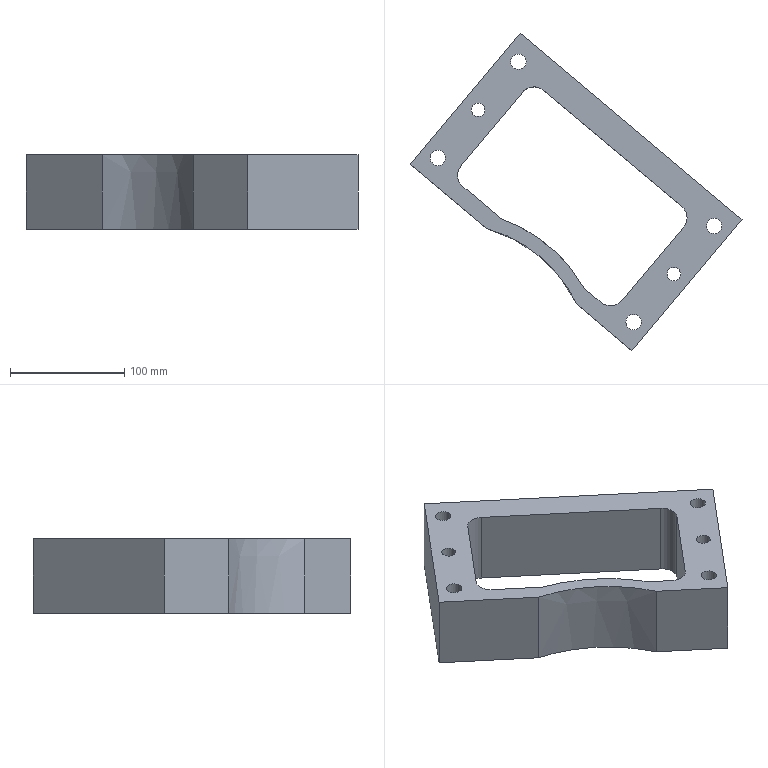Part | NX | features solid 2 | 1 solid | 32 faces | box 290.993 x 278.175 x 65 mm | volume 1076201 mm3 | plane 16 | cylinder 14 | spline 2 | commonest cylinder face diameters 13.5 x4 19.5 x4 26 x4 12 x2
STEP:
#1=CARTESIAN_POINT('',(595.572,489.803,65.));
#2=VERTEX_POINT('',#1);
#3=CARTESIAN_POINT('',(595.572,489.803,0.000000024));
#4=VERTEX_POINT('',#3);
#5=CARTESIAN_POINT('',(595.572,489.803,32.5));
#6=DIRECTION('',(0.,0.,1.));
#7=VECTOR('',#6,1000.);
#8=LINE('',#5,#7);
#9=EDGE_CURVE('',#2,#4,#8,.F.);
#10=ORIENTED_EDGE('',*,*,#9,.F.);
#11=CARTESIAN_POINT('',(610.764,477.056,65.));
#12=VERTEX_POINT('',#11);
#13=CARTESIAN_POINT('',(467.513,597.257,65.));
#14=DIRECTION('',(0.766,-0.6428,0.));
#15=VECTOR('',#14,1000.);
#16=LINE('',#13,#15);
#17=EDGE_CURVE('',#2,#12,#16,.T.);
#18=ORIENTED_EDGE('',*,*,#17,.T.);
#19=CARTESIAN_POINT('',(610.764,477.056,0.000000024));
#20=VERTEX_POINT('',#19);
#21=CARTESIAN_POINT('',(610.764,477.056,70.));
#22=DIRECTION('',(0.,0.,-1.));
#23=VECTOR('',#22,1000.);
#24=LINE('',#21,#23);
#25=EDGE_CURVE('',#20,#12,#24,.F.);
#26=ORIENTED_EDGE('',*,*,#25,.F.);
#27=CARTESIAN_POINT('',(467.513,597.257,0.000000024));
#28=DIRECTION('',(-0.766,0.6428,0.));
#29=VECTOR('',#28,1000.);
#30=LINE('',#27,#29);
#31=EDGE_CURVE('',#4,#20,#30,.F.);
#32=ORIENTED_EDGE('',*,*,#31,.F.);
#33=EDGE_LOOP('',(#10,#18,#26,#32));
#34=FACE_BOUND('',#33,.T.);
#35=CARTESIAN_POINT('',(467.513,597.257,70.));
#36=DIRECTION('',(-0.6428,-0.766,0.));
#37=DIRECTION('',(-0.766,0.6428,0.));
#38=AXIS2_PLACEMENT_3D('',#35,#36,#37);
#39=PLANE('',#38);
#40=ADVANCED_FACE('',(#34),#39,.F.);
#41=CARTESIAN_POINT('',(523.703,550.108,0.000000024));
#42=VERTEX_POINT('',#41);
#43=CARTESIAN_POINT('',(523.703,550.108,65.));
#44=VERTEX_POINT('',#43);
#45=CARTESIAN_POINT('',(523.703,550.108,0.000000024));
#46=DIRECTION('',(0.,0.,1.));
#47=VECTOR('',#46,1000.);
#48=LINE('',#45,#47);
#49=EDGE_CURVE('',#42,#44,#48,.T.);
#50=ORIENTED_EDGE('',*,*,#49,.F.);
#51=CARTESIAN_POINT('',(489.728,578.616,0.000000024));
#52=VERTEX_POINT('',#51);
#53=CARTESIAN_POINT('',(467.513,597.257,0.000000024));
#54=DIRECTION('',(-0.766,0.6428,0.));
#55=VECTOR('',#54,1000.);
#56=LINE('',#53,#55);
#57=EDGE_CURVE('',#52,#42,#56,.F.);
#58=ORIENTED_EDGE('',*,*,#57,.F.);
#59=CARTESIAN_POINT('',(489.728,578.616,65.));
#60=VERTEX_POINT('',#59);
#61=CARTESIAN_POINT('',(489.728,578.616,-5.));
#62=DIRECTION('',(0.,0.,-1.));
#63=VECTOR('',#62,1000.);
#64=LINE('',#61,#63);
#65=EDGE_CURVE('',#60,#52,#64,.T.);
#66=ORIENTED_EDGE('',*,*,#65,.F.);
#67=CARTESIAN_POINT('',(467.513,597.257,65.));
#68=DIRECTION('',(0.766,-0.6428,0.));
#69=VECTOR('',#68,1000.);
#70=LINE('',#67,#69);
#71=EDGE_CURVE('',#60,#44,#70,.T.);
#72=ORIENTED_EDGE('',*,*,#71,.T.);
#73=EDGE_LOOP('',(#50,#58,#66,#72));
#74=FACE_BOUND('',#73,.T.);
#75=CARTESIAN_POINT('',(467.513,597.257,70.));
#76=DIRECTION('',(-0.6428,-0.766,0.));
#77=DIRECTION('',(-0.766,0.6428,0.));
#78=AXIS2_PLACEMENT_3D('',#75,#76,#77);
#79=PLANE('',#78);
#80=ADVANCED_FACE('',(#74),#79,.F.);
#81=CARTESIAN_POINT('',(589.775,475.086,0.000000024));
#82=VERTEX_POINT('',#81);
#83=CARTESIAN_POINT('',(589.775,475.086,65.));
#84=VERTEX_POINT('',#83);
#85=CARTESIAN_POINT('',(589.775,475.086,140.));
#86=CARTESIAN_POINT('',(589.775,475.086,125.));
#87=CARTESIAN_POINT('',(589.775,475.086,110.));
#88=CARTESIAN_POINT('',(589.775,475.086,80.));
#89=CARTESIAN_POINT('',(589.775,475.086,65.));
#90=CARTESIAN_POINT('',(589.775,475.086,20.));
#91=CARTESIAN_POINT('',(589.775,475.086,-10.));
#92=CARTESIAN_POINT('',(589.775,475.086,-40.));
#93=B_SPLINE_CURVE_WITH_KNOTS('',3,(#85,#86,#87,#88,#89,#90,#91,#92),.UNSPECIFIED.,.F.,.F.,(4,2,2,4),(0.,0.25,0.5,1.),.UNSPECIFIED.);
#94=EDGE_CURVE('',#82,#84,#93,.F.);
#95=ORIENTED_EDGE('',*,*,#94,.F.);
#96=CARTESIAN_POINT('',(637.892,434.711,0.000000024));
#97=VERTEX_POINT('',#96);
#98=CARTESIAN_POINT('',(565.395,495.543,0.000000024));
#99=DIRECTION('',(-0.766,0.6428,0.));
#100=VECTOR('',#99,1000.);
#101=LINE('',#98,#100);
#102=EDGE_CURVE('',#82,#97,#101,.F.);
#103=ORIENTED_EDGE('',*,*,#102,.T.);
#104=CARTESIAN_POINT('',(637.892,434.711,65.));
#105=VERTEX_POINT('',#104);
#106=CARTESIAN_POINT('',(637.892,434.711,80.));
#107=DIRECTION('',(0.,0.,1.));
#108=VECTOR('',#107,1000.);
#109=LINE('',#106,#108);
#110=EDGE_CURVE('',#97,#105,#109,.T.);
#111=ORIENTED_EDGE('',*,*,#110,.T.);
#112=CARTESIAN_POINT('',(481.236,566.161,65.));
#113=DIRECTION('',(0.766,-0.6428,0.));
#114=VECTOR('',#113,1000.);
#115=LINE('',#112,#114);
#116=EDGE_CURVE('',#84,#105,#115,.T.);
#117=ORIENTED_EDGE('',*,*,#116,.F.);
#118=EDGE_LOOP('',(#95,#103,#111,#117));
#119=FACE_BOUND('',#118,.T.);
#120=CARTESIAN_POINT('',(565.395,495.543,80.));
#121=DIRECTION('',(0.6428,0.766,0.));
#122=DIRECTION('',(0.766,-0.6428,0.));
#123=AXIS2_PLACEMENT_3D('',#120,#121,#122);
#124=PLANE('',#123);
#125=ADVANCED_FACE('',(#119),#124,.F.);
#126=CARTESIAN_POINT('',(510.282,541.788,65.));
#127=VERTEX_POINT('',#126);
#128=CARTESIAN_POINT('',(510.282,541.788,0.000000024));
#129=VERTEX_POINT('',#128);
#130=CARTESIAN_POINT('',(510.282,541.788,80.));
#131=DIRECTION('',(0.,0.,1.));
#132=VECTOR('',#131,1000.);
#133=LINE('',#130,#132);
#134=EDGE_CURVE('',#127,#129,#133,.F.);
#135=ORIENTED_EDGE('',*,*,#134,.F.);
#136=CARTESIAN_POINT('',(443.317,597.979,65.));
#137=VERTEX_POINT('',#136);
#138=CARTESIAN_POINT('',(481.236,566.161,65.));
#139=DIRECTION('',(0.766,-0.6428,0.));
#140=VECTOR('',#139,1000.);
#141=LINE('',#138,#140);
#142=EDGE_CURVE('',#137,#127,#141,.T.);
#143=ORIENTED_EDGE('',*,*,#142,.F.);
#144=CARTESIAN_POINT('',(443.317,597.979,0.000000024));
#145=VERTEX_POINT('',#144);
#146=CARTESIAN_POINT('',(443.317,597.979,80.));
#147=DIRECTION('',(0.,0.,1.));
#148=VECTOR('',#147,1000.);
#149=LINE('',#146,#148);
#150=EDGE_CURVE('',#145,#137,#149,.T.);
#151=ORIENTED_EDGE('',*,*,#150,.F.);
#152=CARTESIAN_POINT('',(565.395,495.543,0.000000024));
#153=DIRECTION('',(-0.766,0.6428,0.));
#154=VECTOR('',#153,1000.);
#155=LINE('',#152,#154);
#156=EDGE_CURVE('',#145,#129,#155,.F.);
#157=ORIENTED_EDGE('',*,*,#156,.T.);
#158=EDGE_LOOP('',(#135,#143,#151,#157));
#159=FACE_BOUND('',#158,.T.);
#160=CARTESIAN_POINT('',(565.395,495.543,80.));
#161=DIRECTION('',(0.6428,0.766,0.));
#162=DIRECTION('',(0.766,-0.6428,0.));
#163=AXIS2_PLACEMENT_3D('',#160,#161,#162);
#164=PLANE('',#163);
#165=ADVANCED_FACE('',(#159),#164,.F.);
#166=CARTESIAN_POINT('',(589.775,475.086,0.000000024));
#167=CARTESIAN_POINT('',(587.836,479.139,0.000000024));
#168=CARTESIAN_POINT('',(583.553,486.985,0.000000024));
#169=CARTESIAN_POINT('',(575.924,498.063,0.000000024));
#170=CARTESIAN_POINT('',(567.159,508.245,0.000000024));
#171=CARTESIAN_POINT('',(557.474,517.317,0.000000024));
#172=CARTESIAN_POINT('',(546.781,525.352,0.000000024));
#173=CARTESIAN_POINT('',(531.331,534.533,0.000000024));
#174=CARTESIAN_POINT('',(518.946,539.404,0.000000024));
#175=CARTESIAN_POINT('',(510.282,541.788,0.000000024));
#176=B_SPLINE_CURVE_WITH_KNOTS('',3,(#166,#167,#168,#169,#170,#171,#172,#173,#174,#175),.UNSPECIFIED.,.F.,.F.,(4,1,1,1,1,1,1,4),(0.,0.0134,0.0268,0.0402,0.0536,0.067,0.0804,0.1072),.UNSPECIFIED.);
#177=EDGE_CURVE('',#82,#129,#176,.T.);
#178=ORIENTED_EDGE('',*,*,#177,.T.);
#179=ORIENTED_EDGE('',*,*,#156,.F.);
#180=CARTESIAN_POINT('',(539.735,712.886,0.000000024));
#181=VERTEX_POINT('',#180);
#182=CARTESIAN_POINT('',(-69.098,-12.692,0.000000024));
#183=DIRECTION('',(0.6428,0.766,0.));
#184=VECTOR('',#183,1000.);
#185=LINE('',#182,#184);
#186=EDGE_CURVE('',#181,#145,#185,.F.);
#187=ORIENTED_EDGE('',*,*,#186,.F.);
#188=CARTESIAN_POINT('',(734.31,549.618,0.000000024));
#189=VERTEX_POINT('',#188);
#190=CARTESIAN_POINT('',(722.819,559.26,0.000000024));
#191=DIRECTION('',(-0.766,0.6428,0.));
#192=VECTOR('',#191,1000.);
#193=LINE('',#190,#192);
#194=EDGE_CURVE('',#189,#181,#193,.T.);
#195=ORIENTED_EDGE('',*,*,#194,.F.);
#196=CARTESIAN_POINT('',(125.478,-175.96,0.000000024));
#197=DIRECTION('',(0.6428,0.766,0.));
#198=VECTOR('',#197,1000.);
#199=LINE('',#196,#198);
#200=EDGE_CURVE('',#189,#97,#199,.F.);
#201=ORIENTED_EDGE('',*,*,#200,.T.);
#202=ORIENTED_EDGE('',*,*,#102,.F.);
#203=EDGE_LOOP('',(#178,#179,#187,#195,#201,#202));
#204=FACE_BOUND('',#203,.T.);
#205=CARTESIAN_POINT('',(523.703,550.108,0.000000024));
#206=CARTESIAN_POINT('',(531.205,547.402,0.000000024));
#207=CARTESIAN_POINT('',(545.792,540.631,0.000000024));
#208=CARTESIAN_POINT('',(565.448,526.903,0.000000024));
#209=CARTESIAN_POINT('',(582.431,509.864,0.000000024));
#210=CARTESIAN_POINT('',(591.599,496.685,0.000000024));
#211=CARTESIAN_POINT('',(595.572,489.803,0.000000024));
#212=B_SPLINE_CURVE_WITH_KNOTS('',3,(#205,#206,#207,#208,#209,#210,#211),.UNSPECIFIED.,.F.,.F.,(4,1,1,1,4),(0.2128,0.2368,0.2608,0.2847,0.3087),.UNSPECIFIED.);
#213=EDGE_CURVE('',#42,#4,#212,.T.);
#214=ORIENTED_EDGE('',*,*,#213,.T.);
#215=ORIENTED_EDGE('',*,*,#31,.T.);
#216=CARTESIAN_POINT('',(629.078,478.658,0.000000024));
#217=VERTEX_POINT('',#216);
#218=CARTESIAN_POINT('',(619.12,487.014,0.000000024));
#219=DIRECTION('',(0.,0.,-1.));
#220=DIRECTION('',(-1.,0.,0.));
#221=AXIS2_PLACEMENT_3D('',#218,#219,#220);
#222=CIRCLE('',#221,13.);
#223=EDGE_CURVE('',#217,#20,#222,.T.);
#224=ORIENTED_EDGE('',*,*,#223,.F.);
#225=CARTESIAN_POINT('',(683.072,543.006,0.000000024));
#226=VERTEX_POINT('',#225);
#227=CARTESIAN_POINT('',(668.931,526.153,0.000000024));
#228=DIRECTION('',(0.6428,0.766,0.));
#229=VECTOR('',#228,1000.);
#230=LINE('',#227,#229);
#231=EDGE_CURVE('',#226,#217,#230,.F.);
#232=ORIENTED_EDGE('',*,*,#231,.F.);
#233=CARTESIAN_POINT('',(681.47,561.321,0.000000024));
#234=VERTEX_POINT('',#233);
#235=CARTESIAN_POINT('',(673.114,551.362,0.000000024));
#236=DIRECTION('',(0.,0.,-1.));
#237=DIRECTION('',(-1.,0.,0.));
#238=AXIS2_PLACEMENT_3D('',#235,#236,#237);
#239=CIRCLE('',#238,13.);
#240=EDGE_CURVE('',#234,#226,#239,.T.);
#241=ORIENTED_EDGE('',*,*,#240,.F.);
#242=CARTESIAN_POINT('',(560.435,662.881,0.000000024));
#243=VERTEX_POINT('',#242);
#244=CARTESIAN_POINT('',(538.22,681.522,0.000000024));
#245=DIRECTION('',(0.766,-0.6428,0.));
#246=VECTOR('',#245,1000.);
#247=LINE('',#244,#246);
#248=EDGE_CURVE('',#234,#243,#247,.F.);
#249=ORIENTED_EDGE('',*,*,#248,.T.);
#250=CARTESIAN_POINT('',(542.12,661.279,0.000000024));
#251=VERTEX_POINT('',#250);
#252=CARTESIAN_POINT('',(552.079,652.923,0.000000024));
#253=DIRECTION('',(0.,0.,-1.));
#254=DIRECTION('',(-1.,0.,0.));
#255=AXIS2_PLACEMENT_3D('',#252,#253,#254);
#256=CIRCLE('',#255,13.);
#257=EDGE_CURVE('',#251,#243,#256,.T.);
#258=ORIENTED_EDGE('',*,*,#257,.F.);
#259=CARTESIAN_POINT('',(488.126,596.931,0.000000024));
#260=VERTEX_POINT('',#259);
#261=CARTESIAN_POINT('',(527.979,644.426,0.000000024));
#262=DIRECTION('',(0.6428,0.766,0.));
#263=VECTOR('',#262,1000.);
#264=LINE('',#261,#263);
#265=EDGE_CURVE('',#251,#260,#264,.F.);
#266=ORIENTED_EDGE('',*,*,#265,.T.);
#267=CARTESIAN_POINT('',(498.085,588.575,0.000000024));
#268=DIRECTION('',(0.,0.,-1.));
#269=DIRECTION('',(-1.,0.,0.));
#270=AXIS2_PLACEMENT_3D('',#267,#268,#269);
#271=CIRCLE('',#270,13.);
#272=EDGE_CURVE('',#52,#260,#271,.T.);
#273=ORIENTED_EDGE('',*,*,#272,.F.);
#274=ORIENTED_EDGE('',*,*,#57,.T.);
#275=EDGE_LOOP('',(#214,#215,#224,#232,#241,#249,#258,#266,#273,#274));
#276=FACE_BOUND('',#275,.T.);
#277=CARTESIAN_POINT('',(497.016,645.791,0.000000024));
#278=VERTEX_POINT('',#277);
#279=CARTESIAN_POINT('',(503.016,645.791,0.000000024));
#280=DIRECTION('',(0.,0.,-1.));
#281=DIRECTION('',(-1.,0.,0.));
#282=AXIS2_PLACEMENT_3D('',#279,#280,#281);
#283=CIRCLE('',#282,6.);
#284=EDGE_CURVE('',#278,#278,#283,.T.);
#285=ORIENTED_EDGE('',*,*,#284,.F.);
#286=EDGE_LOOP('',(#285));
#287=FACE_BOUND('',#286,.T.);
#288=CARTESIAN_POINT('',(668.61,501.806,0.000000024));
#289=VERTEX_POINT('',#288);
#290=CARTESIAN_POINT('',(674.61,501.806,0.000000024));
#291=DIRECTION('',(0.,0.,-1.));
#292=DIRECTION('',(-1.,0.,0.));
#293=AXIS2_PLACEMENT_3D('',#290,#291,#292);
#294=CIRCLE('',#293,6.);
#295=EDGE_CURVE('',#289,#289,#294,.T.);
#296=ORIENTED_EDGE('',*,*,#295,.F.);
#297=EDGE_LOOP('',(#296));
#298=FACE_BOUND('',#297,.T.);
#299=CARTESIAN_POINT('',(457.913,603.658,0.000000024));
#300=VERTEX_POINT('',#299);
#301=CARTESIAN_POINT('',(467.663,603.658,0.000000024));
#302=DIRECTION('',(0.,0.,-1.));
#303=DIRECTION('',(-1.,0.,0.));
#304=AXIS2_PLACEMENT_3D('',#301,#302,#303);
#305=CIRCLE('',#304,9.75);
#306=EDGE_CURVE('',#300,#300,#305,.T.);
#307=ORIENTED_EDGE('',*,*,#306,.F.);
#308=EDGE_LOOP('',(#307));
#309=FACE_BOUND('',#308,.T.);
#310=CARTESIAN_POINT('',(528.62,687.923,0.000000024));
#311=VERTEX_POINT('',#310);
#312=CARTESIAN_POINT('',(538.37,687.923,0.000000024));
#313=DIRECTION('',(0.,0.,-1.));
#314=DIRECTION('',(-1.,0.,0.));
#315=AXIS2_PLACEMENT_3D('',#312,#313,#314);
#316=CIRCLE('',#315,9.75);
#317=EDGE_CURVE('',#311,#311,#316,.T.);
#318=ORIENTED_EDGE('',*,*,#317,.F.);
#319=EDGE_LOOP('',(#318));
#320=FACE_BOUND('',#319,.T.);
#321=CARTESIAN_POINT('',(700.214,543.939,0.000000024));
#322=VERTEX_POINT('',#321);
#323=CARTESIAN_POINT('',(709.964,543.939,0.000000024));
#324=DIRECTION('',(0.,0.,-1.));
#325=DIRECTION('',(-1.,0.,0.));
#326=AXIS2_PLACEMENT_3D('',#323,#324,#325);
#327=CIRCLE('',#326,9.75);
#328=EDGE_CURVE('',#322,#322,#327,.T.);
#329=ORIENTED_EDGE('',*,*,#328,.F.);
#330=EDGE_LOOP('',(#329));
#331=FACE_BOUND('',#330,.T.);
#332=CARTESIAN_POINT('',(629.507,459.674,0.000000024));
#333=VERTEX_POINT('',#332);
#334=CARTESIAN_POINT('',(639.257,459.674,0.000000024));
#335=DIRECTION('',(0.,0.,-1.));
#336=DIRECTION('',(-1.,0.,0.));
#337=AXIS2_PLACEMENT_3D('',#334,#335,#336);
#338=CIRCLE('',#337,9.75);
#339=EDGE_CURVE('',#333,#333,#338,.T.);
#340=ORIENTED_EDGE('',*,*,#339,.F.);
#341=EDGE_LOOP('',(#340));
#342=FACE_BOUND('',#341,.T.);
#343=CARTESIAN_POINT('',(515.722,654.71,0.000000024));
#344=DIRECTION('',(0.,0.,1.));
#345=DIRECTION('',(-1.,0.,0.));
#346=AXIS2_PLACEMENT_3D('',#343,#344,#345);
#347=PLANE('',#346);
#348=ADVANCED_FACE('',(#204,#276,#287,#298,#309,#320,#331,#342),#347,.F.);
#349=CARTESIAN_POINT('',(510.282,541.788,65.));
#350=CARTESIAN_POINT('',(514.614,540.596,65.));
#351=CARTESIAN_POINT('',(523.093,537.771,65.));
#352=CARTESIAN_POINT('',(535.323,532.174,65.));
#353=CARTESIAN_POINT('',(546.861,525.292,65.));
#354=CARTESIAN_POINT('',(557.469,517.32,65.));
#355=CARTESIAN_POINT('',(567.232,508.177,65.));
#356=CARTESIAN_POINT('',(578.931,494.535,65.));
#357=CARTESIAN_POINT('',(585.897,483.192,65.));
#358=CARTESIAN_POINT('',(589.775,475.086,65.));
#359=B_SPLINE_CURVE_WITH_KNOTS('',3,(#349,#350,#351,#352,#353,#354,#355,#356,#357,#358),.UNSPECIFIED.,.F.,.F.,(4,1,1,1,1,1,1,4),(0.,0.0134,0.02679,0.04019,0.05359,0.06698,0.08038,0.1072),.UNSPECIFIED.);
#360=EDGE_CURVE('',#127,#84,#359,.T.);
#361=ORIENTED_EDGE('',*,*,#360,.T.);
#362=ORIENTED_EDGE('',*,*,#116,.T.);
#363=CARTESIAN_POINT('',(734.31,549.618,65.));
#364=VERTEX_POINT('',#363);
#365=CARTESIAN_POINT('',(644.32,442.372,65.));
#366=DIRECTION('',(-0.6428,-0.766,0.));
#367=VECTOR('',#366,1000.);
#368=LINE('',#365,#367);
#369=EDGE_CURVE('',#364,#105,#368,.T.);
#370=ORIENTED_EDGE('',*,*,#369,.F.);
#371=CARTESIAN_POINT('',(539.735,712.886,65.));
#372=VERTEX_POINT('',#371);
#373=CARTESIAN_POINT('',(577.654,681.068,65.));
#374=DIRECTION('',(0.766,-0.6428,0.));
#375=VECTOR('',#374,1000.);
#376=LINE('',#373,#375);
#377=EDGE_CURVE('',#364,#372,#376,.F.);
#378=ORIENTED_EDGE('',*,*,#377,.T.);
#379=CARTESIAN_POINT('',(449.744,605.64,65.));
#380=DIRECTION('',(-0.6428,-0.766,0.));
#381=VECTOR('',#380,1000.);
#382=LINE('',#379,#381);
#383=EDGE_CURVE('',#372,#137,#382,.T.);
#384=ORIENTED_EDGE('',*,*,#383,.T.);
#385=ORIENTED_EDGE('',*,*,#142,.T.);
#386=EDGE_LOOP('',(#361,#362,#370,#378,#384,#385));
#387=FACE_BOUND('',#386,.T.);
#388=CARTESIAN_POINT('',(595.572,489.803,65.));
#389=CARTESIAN_POINT('',(591.564,496.744,65.));
#390=CARTESIAN_POINT('',(584.685,506.603,65.));
#391=CARTESIAN_POINT('',(574.009,518.313,65.));
#392=CARTESIAN_POINT('',(556.333,534.575,65.));
#393=CARTESIAN_POINT('',(538.673,544.707,65.));
#394=CARTESIAN_POINT('',(523.703,550.108,65.));
#395=B_SPLINE_CURVE_WITH_KNOTS('',3,(#388,#389,#390,#391,#392,#393,#394),.UNSPECIFIED.,.F.,.F.,(4,1,1,1,4),(0.2301,0.2542,0.2662,0.2782,0.3263),.UNSPECIFIED.);
#396=EDGE_CURVE('',#2,#44,#395,.T.);
#397=ORIENTED_EDGE('',*,*,#396,.T.);
#398=ORIENTED_EDGE('',*,*,#71,.F.);
#399=CARTESIAN_POINT('',(488.126,596.931,65.));
#400=VERTEX_POINT('',#399);
#401=CARTESIAN_POINT('',(498.085,588.575,65.));
#402=DIRECTION('',(0.,0.,-1.));
#403=DIRECTION('',(-1.,0.,0.));
#404=AXIS2_PLACEMENT_3D('',#401,#402,#403);
#405=CIRCLE('',#404,13.);
#406=EDGE_CURVE('',#400,#60,#405,.F.);
#407=ORIENTED_EDGE('',*,*,#406,.F.);
#408=CARTESIAN_POINT('',(542.12,661.279,65.));
#409=VERTEX_POINT('',#408);
#410=CARTESIAN_POINT('',(527.979,644.426,65.));
#411=DIRECTION('',(-0.6428,-0.766,0.));
#412=VECTOR('',#411,1000.);
#413=LINE('',#410,#412);
#414=EDGE_CURVE('',#409,#400,#413,.T.);
#415=ORIENTED_EDGE('',*,*,#414,.F.);
#416=CARTESIAN_POINT('',(560.435,662.881,65.));
#417=VERTEX_POINT('',#416);
#418=CARTESIAN_POINT('',(552.079,652.923,65.));
#419=DIRECTION('',(0.,0.,-1.));
#420=DIRECTION('',(-1.,0.,0.));
#421=AXIS2_PLACEMENT_3D('',#418,#419,#420);
#422=CIRCLE('',#421,13.);
#423=EDGE_CURVE('',#417,#409,#422,.F.);
#424=ORIENTED_EDGE('',*,*,#423,.F.);
#425=CARTESIAN_POINT('',(681.47,561.321,65.));
#426=VERTEX_POINT('',#425);
#427=CARTESIAN_POINT('',(538.22,681.522,65.));
#428=DIRECTION('',(-0.766,0.6428,0.));
#429=VECTOR('',#428,1000.);
#430=LINE('',#427,#429);
#431=EDGE_CURVE('',#426,#417,#430,.T.);
#432=ORIENTED_EDGE('',*,*,#431,.F.);
#433=CARTESIAN_POINT('',(683.072,543.006,65.));
#434=VERTEX_POINT('',#433);
#435=CARTESIAN_POINT('',(673.114,551.362,65.));
#436=DIRECTION('',(0.,0.,-1.));
#437=DIRECTION('',(-1.,0.,0.));
#438=AXIS2_PLACEMENT_3D('',#435,#436,#437);
#439=CIRCLE('',#438,13.);
#440=EDGE_CURVE('',#434,#426,#439,.F.);
#441=ORIENTED_EDGE('',*,*,#440,.F.);
#442=CARTESIAN_POINT('',(629.078,478.658,65.));
#443=VERTEX_POINT('',#442);
#444=CARTESIAN_POINT('',(662.503,518.492,65.));
#445=DIRECTION('',(-0.6428,-0.766,0.));
#446=VECTOR('',#445,1000.);
#447=LINE('',#444,#446);
#448=EDGE_CURVE('',#434,#443,#447,.T.);
#449=ORIENTED_EDGE('',*,*,#448,.T.);
#450=CARTESIAN_POINT('',(619.12,487.014,65.));
#451=DIRECTION('',(0.,0.,-1.));
#452=DIRECTION('',(-1.,0.,0.));
#453=AXIS2_PLACEMENT_3D('',#450,#451,#452);
#454=CIRCLE('',#453,13.);
#455=EDGE_CURVE('',#12,#443,#454,.F.);
#456=ORIENTED_EDGE('',*,*,#455,.F.);
#457=ORIENTED_EDGE('',*,*,#17,.F.);
#458=EDGE_LOOP('',(#397,#398,#407,#415,#424,#432,#441,#449,#456,#457));
#459=FACE_BOUND('',#458,.T.);
#460=CARTESIAN_POINT('',(497.016,645.791,65.));
#461=VERTEX_POINT('',#460);
#462=CARTESIAN_POINT('',(503.016,645.791,65.));
#463=DIRECTION('',(0.,0.,-1.));
#464=DIRECTION('',(-1.,0.,0.));
#465=AXIS2_PLACEMENT_3D('',#462,#463,#464);
#466=CIRCLE('',#465,6.);
#467=EDGE_CURVE('',#461,#461,#466,.T.);
#468=ORIENTED_EDGE('',*,*,#467,.T.);
#469=EDGE_LOOP('',(#468));
#470=FACE_BOUND('',#469,.T.);
#471=CARTESIAN_POINT('',(668.61,501.806,65.));
#472=VERTEX_POINT('',#471);
#473=CARTESIAN_POINT('',(674.61,501.806,65.));
#474=DIRECTION('',(0.,0.,-1.));
#475=DIRECTION('',(-1.,0.,0.));
#476=AXIS2_PLACEMENT_3D('',#473,#474,#475);
#477=CIRCLE('',#476,6.);
#478=EDGE_CURVE('',#472,#472,#477,.T.);
#479=ORIENTED_EDGE('',*,*,#478,.T.);
#480=EDGE_LOOP('',(#479));
#481=FACE_BOUND('',#480,.T.);
#482=CARTESIAN_POINT('',(460.913,603.658,65.));
#483=VERTEX_POINT('',#482);
#484=CARTESIAN_POINT('',(467.663,603.658,65.));
#485=DIRECTION('',(0.,0.,-1.));
#486=DIRECTION('',(-1.,0.,0.));
#487=AXIS2_PLACEMENT_3D('',#484,#485,#486);
#488=CIRCLE('',#487,6.75);
#489=EDGE_CURVE('',#483,#483,#488,.T.);
#490=ORIENTED_EDGE('',*,*,#489,.T.);
#491=EDGE_LOOP('',(#490));
#492=FACE_BOUND('',#491,.T.);
#493=CARTESIAN_POINT('',(531.62,687.923,65.));
#494=VERTEX_POINT('',#493);
#495=CARTESIAN_POINT('',(538.37,687.923,65.));
#496=DIRECTION('',(0.,0.,-1.));
#497=DIRECTION('',(-1.,0.,0.));
#498=AXIS2_PLACEMENT_3D('',#495,#496,#497);
#499=CIRCLE('',#498,6.75);
#500=EDGE_CURVE('',#494,#494,#499,.T.);
#501=ORIENTED_EDGE('',*,*,#500,.T.);
#502=EDGE_LOOP('',(#501));
#503=FACE_BOUND('',#502,.T.);
#504=CARTESIAN_POINT('',(703.214,543.939,65.));
#505=VERTEX_POINT('',#504);
#506=CARTESIAN_POINT('',(709.964,543.939,65.));
#507=DIRECTION('',(0.,0.,-1.));
#508=DIRECTION('',(-1.,0.,0.));
#509=AXIS2_PLACEMENT_3D('',#506,#507,#508);
#510=CIRCLE('',#509,6.75);
#511=EDGE_CURVE('',#505,#505,#510,.T.);
#512=ORIENTED_EDGE('',*,*,#511,.T.);
#513=EDGE_LOOP('',(#512));
#514=FACE_BOUND('',#513,.T.);
#515=CARTESIAN_POINT('',(632.507,459.674,65.));
#516=VERTEX_POINT('',#515);
#517=CARTESIAN_POINT('',(639.257,459.674,65.));
#518=DIRECTION('',(0.,0.,-1.));
#519=DIRECTION('',(-1.,0.,0.));
#520=AXIS2_PLACEMENT_3D('',#517,#518,#519);
#521=CIRCLE('',#520,6.75);
#522=EDGE_CURVE('',#516,#516,#521,.T.);
#523=ORIENTED_EDGE('',*,*,#522,.T.);
#524=EDGE_LOOP('',(#523));
#525=FACE_BOUND('',#524,.T.);
#526=CARTESIAN_POINT('',(487.664,573.822,65.));
#527=DIRECTION('',(0.,0.,1.));
#528=DIRECTION('',(0.08716,-0.9962,0.));
#529=AXIS2_PLACEMENT_3D('',#526,#527,#528);
#530=PLANE('',#529);
#531=ADVANCED_FACE('',(#387,#459,#470,#481,#492,#503,#514,#525),#530,.T.);
#532=ORIENTED_EDGE('',*,*,#377,.F.);
#533=CARTESIAN_POINT('',(734.31,549.618,80.));
#534=DIRECTION('',(0.,0.,-1.));
#535=VECTOR('',#534,1000.);
#536=LINE('',#533,#535);
#537=EDGE_CURVE('',#189,#364,#536,.F.);
#538=ORIENTED_EDGE('',*,*,#537,.F.);
#539=ORIENTED_EDGE('',*,*,#194,.T.);
#540=CARTESIAN_POINT('',(539.735,712.886,80.));
#541=DIRECTION('',(0.,0.,-1.));
#542=VECTOR('',#541,1000.);
#543=LINE('',#540,#542);
#544=EDGE_CURVE('',#181,#372,#543,.F.);
#545=ORIENTED_EDGE('',*,*,#544,.T.);
#546=EDGE_LOOP('',(#532,#538,#539,#545));
#547=FACE_BOUND('',#546,.T.);
#548=CARTESIAN_POINT('',(722.819,559.26,0.000000024));
#549=DIRECTION('',(0.6428,0.766,0.));
#550=DIRECTION('',(0.766,-0.6428,0.));
#551=AXIS2_PLACEMENT_3D('',#548,#549,#550);
#552=PLANE('',#551);
#553=ADVANCED_FACE('',(#547),#552,.T.);
#554=ORIENTED_EDGE('',*,*,#110,.F.);
#555=ORIENTED_EDGE('',*,*,#200,.F.);
#556=ORIENTED_EDGE('',*,*,#537,.T.);
#557=ORIENTED_EDGE('',*,*,#369,.T.);
#558=EDGE_LOOP('',(#554,#555,#556,#557));
#559=FACE_BOUND('',#558,.T.);
#560=CARTESIAN_POINT('',(125.478,-175.96,80.));
#561=DIRECTION('',(0.766,-0.6428,0.));
#562=DIRECTION('',(-0.6428,-0.766,0.));
#563=AXIS2_PLACEMENT_3D('',#560,#561,#562);
#564=PLANE('',#563);
#565=ADVANCED_FACE('',(#559),#564,.T.);
#566=ORIENTED_EDGE('',*,*,#544,.F.);
#567=ORIENTED_EDGE('',*,*,#186,.T.);
#568=ORIENTED_EDGE('',*,*,#150,.T.);
#569=ORIENTED_EDGE('',*,*,#383,.F.);
#570=EDGE_LOOP('',(#566,#567,#568,#569));
#571=FACE_BOUND('',#570,.T.);
#572=CARTESIAN_POINT('',(-69.098,-12.692,80.));
#573=DIRECTION('',(0.766,-0.6428,0.));
#574=DIRECTION('',(-0.6428,-0.766,0.));
#575=AXIS2_PLACEMENT_3D('',#572,#573,#574);
#576=PLANE('',#575);
#577=ADVANCED_FACE('',(#571),#576,.F.);
#578=ORIENTED_EDGE('',*,*,#231,.T.);
#579=CARTESIAN_POINT('',(629.078,478.658,100.));
#580=DIRECTION('',(0.,0.,-1.));
#581=VECTOR('',#580,1000.);
#582=LINE('',#579,#581);
#583=EDGE_CURVE('',#443,#217,#582,.T.);
#584=ORIENTED_EDGE('',*,*,#583,.F.);
#585=ORIENTED_EDGE('',*,*,#448,.F.);
#586=CARTESIAN_POINT('',(683.072,543.006,100.));
#587=DIRECTION('',(0.,0.,-1.));
#588=VECTOR('',#587,1000.);
#589=LINE('',#586,#588);
#590=EDGE_CURVE('',#226,#434,#589,.F.);
#591=ORIENTED_EDGE('',*,*,#590,.F.);
#592=EDGE_LOOP('',(#578,#584,#585,#591));
#593=FACE_BOUND('',#592,.T.);
#594=CARTESIAN_POINT('',(662.503,518.492,100.));
#595=DIRECTION('',(-0.766,0.6428,0.));
#596=DIRECTION('',(-0.6428,-0.766,0.));
#597=AXIS2_PLACEMENT_3D('',#594,#595,#596);
#598=PLANE('',#597);
#599=ADVANCED_FACE('',(#593),#598,.T.);
#600=ORIENTED_EDGE('',*,*,#414,.T.);
#601=CARTESIAN_POINT('',(488.126,596.931,80.));
#602=DIRECTION('',(0.,0.,-1.));
#603=VECTOR('',#602,1000.);
#604=LINE('',#601,#603);
#605=EDGE_CURVE('',#260,#400,#604,.F.);
#606=ORIENTED_EDGE('',*,*,#605,.F.);
#607=ORIENTED_EDGE('',*,*,#265,.F.);
#608=CARTESIAN_POINT('',(542.12,661.279,-5.));
#609=DIRECTION('',(0.,0.,-1.));
#610=VECTOR('',#609,1000.);
#611=LINE('',#608,#610);
#612=EDGE_CURVE('',#409,#251,#611,.T.);
#613=ORIENTED_EDGE('',*,*,#612,.F.);
#614=EDGE_LOOP('',(#600,#606,#607,#613));
#615=FACE_BOUND('',#614,.T.);
#616=CARTESIAN_POINT('',(527.979,644.426,0.000000024));
#617=DIRECTION('',(-0.766,0.6428,0.));
#618=DIRECTION('',(0.6428,0.766,0.));
#619=AXIS2_PLACEMENT_3D('',#616,#617,#618);
#620=PLANE('',#619);
#621=ADVANCED_FACE('',(#615),#620,.F.);
#622=ORIENTED_EDGE('',*,*,#248,.F.);
#623=CARTESIAN_POINT('',(681.47,561.321,70.));
#624=DIRECTION('',(0.,0.,-1.));
#625=VECTOR('',#624,1000.);
#626=LINE('',#623,#625);
#627=EDGE_CURVE('',#426,#234,#626,.T.);
#628=ORIENTED_EDGE('',*,*,#627,.F.);
#629=ORIENTED_EDGE('',*,*,#431,.T.);
#630=CARTESIAN_POINT('',(560.435,662.881,80.));
#631=DIRECTION('',(0.,0.,-1.));
#632=VECTOR('',#631,1000.);
#633=LINE('',#630,#632);
#634=EDGE_CURVE('',#243,#417,#633,.F.);
#635=ORIENTED_EDGE('',*,*,#634,.F.);
#636=EDGE_LOOP('',(#622,#628,#629,#635));
#637=FACE_BOUND('',#636,.T.);
#638=CARTESIAN_POINT('',(538.22,681.522,70.));
#639=DIRECTION('',(0.6428,0.766,0.));
#640=DIRECTION('',(0.766,-0.6428,0.));
#641=AXIS2_PLACEMENT_3D('',#638,#639,#640);
#642=PLANE('',#641);
#643=ADVANCED_FACE('',(#637),#642,.F.);
#644=ORIENTED_EDGE('',*,*,#423,.T.);
#645=ORIENTED_EDGE('',*,*,#612,.T.);
#646=ORIENTED_EDGE('',*,*,#257,.T.);
#647=ORIENTED_EDGE('',*,*,#634,.T.);
#648=EDGE_LOOP('',(#644,#645,#646,#647));
#649=FACE_BOUND('',#648,.T.);
#650=CARTESIAN_POINT('',(552.079,652.923,0.000000024));
#651=DIRECTION('',(0.,0.,1.));
#652=DIRECTION('',(-1.,0.,0.));
#653=AXIS2_PLACEMENT_3D('',#650,#651,#652);
#654=CYLINDRICAL_SURFACE('',#653,13.);
#655=ADVANCED_FACE('',(#649),#654,.F.);
#656=ORIENTED_EDGE('',*,*,#440,.T.);
#657=ORIENTED_EDGE('',*,*,#627,.T.);
#658=ORIENTED_EDGE('',*,*,#240,.T.);
#659=ORIENTED_EDGE('',*,*,#590,.T.);
#660=EDGE_LOOP('',(#656,#657,#658,#659));
#661=FACE_BOUND('',#660,.T.);
#662=CARTESIAN_POINT('',(673.114,551.362,70.));
#663=DIRECTION('',(0.,0.,-1.));
#664=DIRECTION('',(1.,0.,0.));
#665=AXIS2_PLACEMENT_3D('',#662,#663,#664);
#666=CYLINDRICAL_SURFACE('',#665,13.);
#667=ADVANCED_FACE('',(#661),#666,.F.);
#668=ORIENTED_EDGE('',*,*,#455,.T.);
#669=ORIENTED_EDGE('',*,*,#583,.T.);
#670=ORIENTED_EDGE('',*,*,#223,.T.);
#671=ORIENTED_EDGE('',*,*,#25,.T.);
#672=EDGE_LOOP('',(#668,#669,#670,#671));
#673=FACE_BOUND('',#672,.T.);
#674=CARTESIAN_POINT('',(619.12,487.014,100.));
#675=DIRECTION('',(0.,0.,-1.));
#676=DIRECTION('',(1.,0.,0.));
#677=AXIS2_PLACEMENT_3D('',#674,#675,#676);
#678=CYLINDRICAL_SURFACE('',#677,13.);
#679=ADVANCED_FACE('',(#673),#678,.F.);
#680=ORIENTED_EDGE('',*,*,#406,.T.);
#681=ORIENTED_EDGE('',*,*,#65,.T.);
#682=ORIENTED_EDGE('',*,*,#272,.T.);
#683=ORIENTED_EDGE('',*,*,#605,.T.);
#684=EDGE_LOOP('',(#680,#681,#682,#683));
#685=FACE_BOUND('',#684,.T.);
#686=CARTESIAN_POINT('',(498.085,588.575,70.));
#687=DIRECTION('',(0.,0.,1.));
#688=DIRECTION('',(-1.,0.,0.));
#689=AXIS2_PLACEMENT_3D('',#686,#687,#688);
#690=CYLINDRICAL_SURFACE('',#689,13.);
#691=ADVANCED_FACE('',(#685),#690,.F.);
#692=ORIENTED_EDGE('',*,*,#522,.F.);
#693=EDGE_LOOP('',(#692));
#694=FACE_BOUND('',#693,.T.);
#695=CARTESIAN_POINT('',(632.507,459.674,40.));
#696=VERTEX_POINT('',#695);
#697=CARTESIAN_POINT('',(639.257,459.674,40.));
#698=DIRECTION('',(0.,0.,-1.));
#699=DIRECTION('',(-1.,0.,0.));
#700=AXIS2_PLACEMENT_3D('',#697,#698,#699);
#701=CIRCLE('',#700,6.75);
#702=EDGE_CURVE('',#696,#696,#701,.T.);
#703=ORIENTED_EDGE('',*,*,#702,.T.);
#704=EDGE_LOOP('',(#703));
#705=FACE_BOUND('',#704,.T.);
#706=CARTESIAN_POINT('',(639.257,459.674,95.));
#707=DIRECTION('',(0.,0.,1.));
#708=DIRECTION('',(-1.,0.,0.));
#709=AXIS2_PLACEMENT_3D('',#706,#707,#708);
#710=CYLINDRICAL_SURFACE('',#709,6.75);
#711=ADVANCED_FACE('',(#694,#705),#710,.F.);
#712=ORIENTED_EDGE('',*,*,#702,.F.);
#713=EDGE_LOOP('',(#712));
#714=FACE_BOUND('',#713,.T.);
#715=CARTESIAN_POINT('',(629.507,459.674,40.));
#716=VERTEX_POINT('',#715);
#717=CARTESIAN_POINT('',(639.257,459.674,40.));
#718=DIRECTION('',(0.,0.,-1.));
#719=DIRECTION('',(-1.,0.,0.));
#720=AXIS2_PLACEMENT_3D('',#717,#718,#719);
#721=CIRCLE('',#720,9.75);
#722=EDGE_CURVE('',#716,#716,#721,.T.);
#723=ORIENTED_EDGE('',*,*,#722,.T.);
#724=EDGE_LOOP('',(#723));
#725=FACE_BOUND('',#724,.T.);
#726=CARTESIAN_POINT('',(639.257,459.674,40.));
#727=DIRECTION('',(0.,0.,1.));
#728=DIRECTION('',(-1.,0.,0.));
#729=AXIS2_PLACEMENT_3D('',#726,#727,#728);
#730=PLANE('',#729);
#731=ADVANCED_FACE('',(#714,#725),#730,.F.);
#732=ORIENTED_EDGE('',*,*,#722,.F.);
#733=EDGE_LOOP('',(#732));
#734=FACE_BOUND('',#733,.T.);
#735=ORIENTED_EDGE('',*,*,#339,.T.);
#736=EDGE_LOOP('',(#735));
#737=FACE_BOUND('',#736,.T.);
#738=CARTESIAN_POINT('',(639.257,459.674,-5.));
#739=DIRECTION('',(0.,0.,1.));
#740=DIRECTION('',(-1.,0.,0.));
#741=AXIS2_PLACEMENT_3D('',#738,#739,#740);
#742=CYLINDRICAL_SURFACE('',#741,9.75);
#743=ADVANCED_FACE('',(#734,#737),#742,.F.);
#744=ORIENTED_EDGE('',*,*,#511,.F.);
#745=EDGE_LOOP('',(#744));
#746=FACE_BOUND('',#745,.T.);
#747=CARTESIAN_POINT('',(703.214,543.939,40.));
#748=VERTEX_POINT('',#747);
#749=CARTESIAN_POINT('',(709.964,543.939,40.));
#750=DIRECTION('',(0.,0.,-1.));
#751=DIRECTION('',(-1.,0.,0.));
#752=AXIS2_PLACEMENT_3D('',#749,#750,#751);
#753=CIRCLE('',#752,6.75);
#754=EDGE_CURVE('',#748,#748,#753,.T.);
#755=ORIENTED_EDGE('',*,*,#754,.T.);
#756=EDGE_LOOP('',(#755));
#757=FACE_BOUND('',#756,.T.);
#758=CARTESIAN_POINT('',(709.964,543.939,95.));
#759=DIRECTION('',(0.,0.,1.));
#760=DIRECTION('',(-1.,0.,0.));
#761=AXIS2_PLACEMENT_3D('',#758,#759,#760);
#762=CYLINDRICAL_SURFACE('',#761,6.75);
#763=ADVANCED_FACE('',(#746,#757),#762,.F.);
#764=ORIENTED_EDGE('',*,*,#754,.F.);
#765=EDGE_LOOP('',(#764));
#766=FACE_BOUND('',#765,.T.);
#767=CARTESIAN_POINT('',(700.214,543.939,40.));
#768=VERTEX_POINT('',#767);
#769=CARTESIAN_POINT('',(709.964,543.939,40.));
#770=DIRECTION('',(0.,0.,-1.));
#771=DIRECTION('',(-1.,0.,0.));
#772=AXIS2_PLACEMENT_3D('',#769,#770,#771);
#773=CIRCLE('',#772,9.75);
#774=EDGE_CURVE('',#768,#768,#773,.T.);
#775=ORIENTED_EDGE('',*,*,#774,.T.);
#776=EDGE_LOOP('',(#775));
#777=FACE_BOUND('',#776,.T.);
#778=CARTESIAN_POINT('',(703.536,536.278,40.));
#779=DIRECTION('',(0.,0.,1.));
#780=DIRECTION('',(-1.,0.,0.));
#781=AXIS2_PLACEMENT_3D('',#778,#779,#780);
#782=PLANE('',#781);
#783=ADVANCED_FACE('',(#766,#777),#782,.F.);
#784=ORIENTED_EDGE('',*,*,#774,.F.);
#785=EDGE_LOOP('',(#784));
#786=FACE_BOUND('',#785,.T.);
#787=ORIENTED_EDGE('',*,*,#328,.T.);
#788=EDGE_LOOP('',(#787));
#789=FACE_BOUND('',#788,.T.);
#790=CARTESIAN_POINT('',(709.964,543.939,-5.));
#791=DIRECTION('',(0.,0.,1.));
#792=DIRECTION('',(-1.,0.,0.));
#793=AXIS2_PLACEMENT_3D('',#790,#791,#792);
#794=CYLINDRICAL_SURFACE('',#793,9.75);
#795=ADVANCED_FACE('',(#786,#789),#794,.F.);
#796=ORIENTED_EDGE('',*,*,#500,.F.);
#797=EDGE_LOOP('',(#796));
#798=FACE_BOUND('',#797,.T.);
#799=CARTESIAN_POINT('',(531.62,687.923,40.));
#800=VERTEX_POINT('',#799);
#801=CARTESIAN_POINT('',(538.37,687.923,40.));
#802=DIRECTION('',(0.,0.,-1.));
#803=DIRECTION('',(-1.,0.,0.));
#804=AXIS2_PLACEMENT_3D('',#801,#802,#803);
#805=CIRCLE('',#804,6.75);
#806=EDGE_CURVE('',#800,#800,#805,.T.);
#807=ORIENTED_EDGE('',*,*,#806,.T.);
#808=EDGE_LOOP('',(#807));
#809=FACE_BOUND('',#808,.T.);
#810=CARTESIAN_POINT('',(538.37,687.923,95.));
#811=DIRECTION('',(0.,0.,1.));
#812=DIRECTION('',(-1.,0.,0.));
#813=AXIS2_PLACEMENT_3D('',#810,#811,#812);
#814=CYLINDRICAL_SURFACE('',#813,6.75);
#815=ADVANCED_FACE('',(#798,#809),#814,.F.);
#816=ORIENTED_EDGE('',*,*,#806,.F.);
#817=EDGE_LOOP('',(#816));
#818=FACE_BOUND('',#817,.T.);
#819=CARTESIAN_POINT('',(528.62,687.923,40.));
#820=VERTEX_POINT('',#819);
#821=CARTESIAN_POINT('',(538.37,687.923,40.));
#822=DIRECTION('',(0.,0.,-1.));
#823=DIRECTION('',(-1.,0.,0.));
#824=AXIS2_PLACEMENT_3D('',#821,#822,#823);
#825=CIRCLE('',#824,9.75);
#826=EDGE_CURVE('',#820,#820,#825,.T.);
#827=ORIENTED_EDGE('',*,*,#826,.T.);
#828=EDGE_LOOP('',(#827));
#829=FACE_BOUND('',#828,.T.);
#830=CARTESIAN_POINT('',(531.942,680.263,40.));
#831=DIRECTION('',(0.,0.,1.));
#832=DIRECTION('',(-1.,0.,0.));
#833=AXIS2_PLACEMENT_3D('',#830,#831,#832);
#834=PLANE('',#833);
#835=ADVANCED_FACE('',(#818,#829),#834,.F.);
#836=ORIENTED_EDGE('',*,*,#826,.F.);
#837=EDGE_LOOP('',(#836));
#838=FACE_BOUND('',#837,.T.);
#839=ORIENTED_EDGE('',*,*,#317,.T.);
#840=EDGE_LOOP('',(#839));
#841=FACE_BOUND('',#840,.T.);
#842=CARTESIAN_POINT('',(538.37,687.923,-5.));
#843=DIRECTION('',(0.,0.,1.));
#844=DIRECTION('',(-1.,0.,0.));
#845=AXIS2_PLACEMENT_3D('',#842,#843,#844);
#846=CYLINDRICAL_SURFACE('',#845,9.75);
#847=ADVANCED_FACE('',(#838,#841),#846,.F.);
#848=ORIENTED_EDGE('',*,*,#489,.F.);
#849=EDGE_LOOP('',(#848));
#850=FACE_BOUND('',#849,.T.);
#851=CARTESIAN_POINT('',(460.913,603.658,40.));
#852=VERTEX_POINT('',#851);
#853=CARTESIAN_POINT('',(467.663,603.658,40.));
#854=DIRECTION('',(0.,0.,-1.));
#855=DIRECTION('',(-1.,0.,0.));
#856=AXIS2_PLACEMENT_3D('',#853,#854,#855);
#857=CIRCLE('',#856,6.75);
#858=EDGE_CURVE('',#852,#852,#857,.T.);
#859=ORIENTED_EDGE('',*,*,#858,.T.);
#860=EDGE_LOOP('',(#859));
#861=FACE_BOUND('',#860,.T.);
#862=CARTESIAN_POINT('',(467.663,603.658,95.));
#863=DIRECTION('',(0.,0.,1.));
#864=DIRECTION('',(-1.,0.,0.));
#865=AXIS2_PLACEMENT_3D('',#862,#863,#864);
#866=CYLINDRICAL_SURFACE('',#865,6.75);
#867=ADVANCED_FACE('',(#850,#861),#866,.F.);
#868=ORIENTED_EDGE('',*,*,#858,.F.);
#869=EDGE_LOOP('',(#868));
#870=FACE_BOUND('',#869,.T.);
#871=CARTESIAN_POINT('',(457.913,603.658,40.));
#872=VERTEX_POINT('',#871);
#873=CARTESIAN_POINT('',(467.663,603.658,40.));
#874=DIRECTION('',(0.,0.,-1.));
#875=DIRECTION('',(-1.,0.,0.));
#876=AXIS2_PLACEMENT_3D('',#873,#874,#875);
#877=CIRCLE('',#876,9.75);
#878=EDGE_CURVE('',#872,#872,#877,.T.);
#879=ORIENTED_EDGE('',*,*,#878,.T.);
#880=EDGE_LOOP('',(#879));
#881=FACE_BOUND('',#880,.T.);
#882=CARTESIAN_POINT('',(467.663,603.658,40.));
#883=DIRECTION('',(0.,0.,1.));
#884=DIRECTION('',(-1.,0.,0.));
#885=AXIS2_PLACEMENT_3D('',#882,#883,#884);
#886=PLANE('',#885);
#887=ADVANCED_FACE('',(#870,#881),#886,.F.);
#888=ORIENTED_EDGE('',*,*,#878,.F.);
#889=EDGE_LOOP('',(#888));
#890=FACE_BOUND('',#889,.T.);
#891=ORIENTED_EDGE('',*,*,#306,.T.);
#892=EDGE_LOOP('',(#891));
#893=FACE_BOUND('',#892,.T.);
#894=CARTESIAN_POINT('',(467.663,603.658,-5.));
#895=DIRECTION('',(0.,0.,1.));
#896=DIRECTION('',(-1.,0.,0.));
#897=AXIS2_PLACEMENT_3D('',#894,#895,#896);
#898=CYLINDRICAL_SURFACE('',#897,9.75);
#899=ADVANCED_FACE('',(#890,#893),#898,.F.);
#900=ORIENTED_EDGE('',*,*,#478,.F.);
#901=EDGE_LOOP('',(#900));
#902=FACE_BOUND('',#901,.T.);
#903=ORIENTED_EDGE('',*,*,#295,.T.);
#904=EDGE_LOOP('',(#903));
#905=FACE_BOUND('',#904,.T.);
#906=CARTESIAN_POINT('',(674.61,501.806,-5.));
#907=DIRECTION('',(0.,0.,1.));
#908=DIRECTION('',(-1.,0.,0.));
#909=AXIS2_PLACEMENT_3D('',#906,#907,#908);
#910=CYLINDRICAL_SURFACE('',#909,6.);
#911=ADVANCED_FACE('',(#902,#905),#910,.F.);
#912=ORIENTED_EDGE('',*,*,#467,.F.);
#913=EDGE_LOOP('',(#912));
#914=FACE_BOUND('',#913,.T.);
#915=ORIENTED_EDGE('',*,*,#284,.T.);
#916=EDGE_LOOP('',(#915));
#917=FACE_BOUND('',#916,.T.);
#918=CARTESIAN_POINT('',(503.016,645.791,-5.));
#919=DIRECTION('',(0.,0.,1.));
#920=DIRECTION('',(-1.,0.,0.));
#921=AXIS2_PLACEMENT_3D('',#918,#919,#920);
#922=CYLINDRICAL_SURFACE('',#921,6.);
#923=ADVANCED_FACE('',(#914,#917),#922,.F.);
#924=ORIENTED_EDGE('',*,*,#94,.T.);
#925=ORIENTED_EDGE('',*,*,#360,.F.);
#926=ORIENTED_EDGE('',*,*,#134,.T.);
#927=ORIENTED_EDGE('',*,*,#177,.F.);
#928=EDGE_LOOP('',(#924,#925,#926,#927));
#929=FACE_BOUND('',#928,.T.);
#930=CARTESIAN_POINT('',(589.775,475.086,65.));
#931=CARTESIAN_POINT('',(589.775,475.086,60.));
#932=CARTESIAN_POINT('',(589.775,475.086,55.));
#933=CARTESIAN_POINT('',(589.775,475.086,33.333));
#934=CARTESIAN_POINT('',(589.775,475.086,16.667));
#935=CARTESIAN_POINT('',(589.775,475.086,0.000000024));
#936=CARTESIAN_POINT('',(586.046,482.881,65.));
#937=CARTESIAN_POINT('',(586.046,482.881,60.));
#938=CARTESIAN_POINT('',(586.046,482.881,55.));
#939=CARTESIAN_POINT('',(586.046,482.881,33.333));
#940=CARTESIAN_POINT('',(586.046,482.881,16.667));
#941=CARTESIAN_POINT('',(586.046,482.881,0.000000024));
#942=CARTESIAN_POINT('',(581.377,490.558,65.));
#943=CARTESIAN_POINT('',(581.377,490.558,60.));
#944=CARTESIAN_POINT('',(581.377,490.558,55.));
#945=CARTESIAN_POINT('',(581.377,490.558,33.333));
#946=CARTESIAN_POINT('',(581.377,490.558,16.667));
#947=CARTESIAN_POINT('',(581.377,490.558,0.000000024));
#948=CARTESIAN_POINT('',(575.957,497.625,65.));
#949=CARTESIAN_POINT('',(575.957,497.625,60.));
#950=CARTESIAN_POINT('',(575.957,497.625,55.));
#951=CARTESIAN_POINT('',(575.957,497.625,33.333));
#952=CARTESIAN_POINT('',(575.957,497.625,16.667));
#953=CARTESIAN_POINT('',(575.957,497.625,0.000000024));
#954=CARTESIAN_POINT('',(570.536,504.692,65.));
#955=CARTESIAN_POINT('',(570.536,504.692,60.));
#956=CARTESIAN_POINT('',(570.536,504.692,55.));
#957=CARTESIAN_POINT('',(570.536,504.692,33.333));
#958=CARTESIAN_POINT('',(570.536,504.692,16.667));
#959=CARTESIAN_POINT('',(570.536,504.692,0.000000024));
#960=CARTESIAN_POINT('',(564.397,511.163,65.));
#961=CARTESIAN_POINT('',(564.397,511.163,60.));
#962=CARTESIAN_POINT('',(564.397,511.163,55.));
#963=CARTESIAN_POINT('',(564.397,511.163,33.333));
#964=CARTESIAN_POINT('',(564.397,511.163,16.667));
#965=CARTESIAN_POINT('',(564.397,511.163,0.000000024));
#966=CARTESIAN_POINT('',(557.493,516.986,65.));
#967=CARTESIAN_POINT('',(557.493,516.986,60.));
#968=CARTESIAN_POINT('',(557.493,516.986,55.));
#969=CARTESIAN_POINT('',(557.493,516.986,33.333));
#970=CARTESIAN_POINT('',(557.493,516.986,16.667));
#971=CARTESIAN_POINT('',(557.493,516.986,0.000000024));
#972=CARTESIAN_POINT('',(550.59,522.81,65.));
#973=CARTESIAN_POINT('',(550.59,522.81,60.));
#974=CARTESIAN_POINT('',(550.59,522.81,55.));
#975=CARTESIAN_POINT('',(550.59,522.81,33.333));
#976=CARTESIAN_POINT('',(550.59,522.81,16.667));
#977=CARTESIAN_POINT('',(550.59,522.81,0.000000024));
#978=CARTESIAN_POINT('',(543.012,527.871,65.));
#979=CARTESIAN_POINT('',(543.012,527.871,60.));
#980=CARTESIAN_POINT('',(543.012,527.871,55.));
#981=CARTESIAN_POINT('',(543.012,527.871,33.333));
#982=CARTESIAN_POINT('',(543.012,527.871,16.667));
#983=CARTESIAN_POINT('',(543.012,527.871,0.000000024));
#984=CARTESIAN_POINT('',(535.146,531.992,65.));
#985=CARTESIAN_POINT('',(535.146,531.992,60.));
#986=CARTESIAN_POINT('',(535.146,531.992,55.));
#987=CARTESIAN_POINT('',(535.146,531.992,33.333));
#988=CARTESIAN_POINT('',(535.146,531.992,16.667));
#989=CARTESIAN_POINT('',(535.146,531.992,0.000000024));
#990=CARTESIAN_POINT('',(531.213,534.053,65.));
#991=CARTESIAN_POINT('',(531.213,534.053,60.));
#992=CARTESIAN_POINT('',(531.213,534.053,55.));
#993=CARTESIAN_POINT('',(531.213,534.053,33.333));
#994=CARTESIAN_POINT('',(531.213,534.053,16.667));
#995=CARTESIAN_POINT('',(531.213,534.053,0.000000024));
#996=CARTESIAN_POINT('',(527.158,535.91,65.));
#997=CARTESIAN_POINT('',(527.158,535.91,60.));
#998=CARTESIAN_POINT('',(527.158,535.91,55.));
#999=CARTESIAN_POINT('',(527.158,535.91,33.333));
#1000=CARTESIAN_POINT('',(527.158,535.91,16.667));
#1001=CARTESIAN_POINT('',(527.158,535.91,0.000000024));
#1002=CARTESIAN_POINT('',(523.,537.549,65.));
#1003=CARTESIAN_POINT('',(523.,537.549,60.));
#1004=CARTESIAN_POINT('',(523.,537.549,55.));
#1005=CARTESIAN_POINT('',(523.,537.549,33.333));
#1006=CARTESIAN_POINT('',(523.,537.549,16.667));
#1007=CARTESIAN_POINT('',(523.,537.549,0.000000024));
#1008=CARTESIAN_POINT('',(518.841,539.188,65.));
#1009=CARTESIAN_POINT('',(518.841,539.188,60.));
#1010=CARTESIAN_POINT('',(518.841,539.188,55.));
#1011=CARTESIAN_POINT('',(518.841,539.188,33.333));
#1012=CARTESIAN_POINT('',(518.841,539.188,16.667));
#1013=CARTESIAN_POINT('',(518.841,539.188,0.000000024));
#1014=CARTESIAN_POINT('',(514.549,540.614,65.));
#1015=CARTESIAN_POINT('',(514.549,540.614,60.));
#1016=CARTESIAN_POINT('',(514.549,540.614,55.));
#1017=CARTESIAN_POINT('',(514.549,540.614,33.333));
#1018=CARTESIAN_POINT('',(514.549,540.614,16.667));
#1019=CARTESIAN_POINT('',(514.549,540.614,0.000000024));
#1020=CARTESIAN_POINT('',(510.282,541.788,65.));
#1021=CARTESIAN_POINT('',(510.282,541.788,60.));
#1022=CARTESIAN_POINT('',(510.282,541.788,55.));
#1023=CARTESIAN_POINT('',(510.282,541.788,33.333));
#1024=CARTESIAN_POINT('',(510.282,541.788,16.667));
#1025=CARTESIAN_POINT('',(510.282,541.788,0.000000024));
#1026=B_SPLINE_SURFACE_WITH_KNOTS('',3,3,((#930,#931,#932,#933,#934,#935),(#936,#937,#938,#939,#940,#941),(#942,#943,#944,#945,#946,#947),(#948,#949,#950,#951,#952,#953),(#954,#955,#956,#957,#958,#959),(#960,#961,#962,#963,#964,#965),(#966,#967,#968,#969,#970,#971),(#972,#973,#974,#975,#976,#977),(#978,#979,#980,#981,#982,#983),(#984,#985,#986,#987,#988,#989),(#990,#991,#992,#993,#994,#995),(#996,#997,#998,#999,#1000,#1001),(#1002,#1003,#1004,#1005,#1006,#1007),(#1008,#1009,#1010,#1011,#1012,#1013),(#1014,#1015,#1016,#1017,#1018,#1019),(#1020,#1021,#1022,#1023,#1024,#1025)),.SURF_OF_LINEAR_EXTRUSION.,.F.,.F.,.F.,(4,3,3,3,3,4),(4,2,4),(0.,0.25,0.5,0.75,0.875,1.),(0.4167,0.5,0.7778),.UNSPECIFIED.);
#1027=ADVANCED_FACE('',(#929),#1026,.T.);
#1028=ORIENTED_EDGE('',*,*,#396,.F.);
#1029=ORIENTED_EDGE('',*,*,#9,.T.);
#1030=ORIENTED_EDGE('',*,*,#213,.F.);
#1031=ORIENTED_EDGE('',*,*,#49,.T.);
#1032=EDGE_LOOP('',(#1028,#1029,#1030,#1031));
#1033=FACE_BOUND('',#1032,.T.);
#1034=CARTESIAN_POINT('',(523.703,550.108,0.000000024));
#1035=CARTESIAN_POINT('',(523.703,550.108,65.));
#1036=CARTESIAN_POINT('',(531.233,547.392,0.000000024));
#1037=CARTESIAN_POINT('',(531.233,547.392,65.));
#1038=CARTESIAN_POINT('',(542.036,542.382,0.000000024));
#1039=CARTESIAN_POINT('',(542.036,542.382,65.));
#1040=CARTESIAN_POINT('',(555.597,533.785,0.000000024));
#1041=CARTESIAN_POINT('',(555.597,533.785,65.));
#1042=CARTESIAN_POINT('',(568.47,523.908,0.000000024));
#1043=CARTESIAN_POINT('',(568.47,523.908,65.));
#1044=CARTESIAN_POINT('',(582.535,509.722,0.000000024));
#1045=CARTESIAN_POINT('',(582.535,509.722,65.));
#1046=CARTESIAN_POINT('',(591.647,496.601,0.000000024));
#1047=CARTESIAN_POINT('',(591.647,496.601,65.));
#1048=CARTESIAN_POINT('',(595.572,489.803,0.000000024));
#1049=CARTESIAN_POINT('',(595.572,489.803,65.));
#1050=B_SPLINE_SURFACE_WITH_KNOTS('',3,1,((#1034,#1035),(#1036,#1037),(#1038,#1039),(#1040,#1041),(#1042,#1043),(#1044,#1045),(#1046,#1047),(#1048,#1049)),.SURF_OF_LINEAR_EXTRUSION.,.F.,.F.,.F.,(4,1,1,1,1,4),(2,2),(0.06717,0.283,0.391,0.4989,0.7148,0.9307),(0.,1.),.UNSPECIFIED.);
#1051=ADVANCED_FACE('',(#1033),#1050,.F.);
#1052=CLOSED_SHELL('',(#40,#80,#125,#165,#348,#531,#553,#565,#577,#599,#621,#643,#655,#667,#679,#691,#711,#731,#743,#763,#783,#795,#815,#835,#847,#867,#887,#899,#911,#923,#1027,#1051));
#1053=MANIFOLD_SOLID_BREP('',#1052);
#1054=(LENGTH_UNIT()NAMED_UNIT(*)SI_UNIT(.MILLI.,.METRE.));
#1055=UNCERTAINTY_MEASURE_WITH_UNIT(LENGTH_MEASURE(0.0508),#1054,'','');
#1056=(NAMED_UNIT(*)PLANE_ANGLE_UNIT()SI_UNIT($,.RADIAN.));
#1057=(NAMED_UNIT(*)SI_UNIT($,.STERADIAN.)SOLID_ANGLE_UNIT());
#1058=(GEOMETRIC_REPRESENTATION_CONTEXT(3)GLOBAL_UNCERTAINTY_ASSIGNED_CONTEXT((#1055))GLOBAL_UNIT_ASSIGNED_CONTEXT((#1054,#1056,#1057))REPRESENTATION_CONTEXT('',''));
#1059=ADVANCED_BREP_SHAPE_REPRESENTATION('',(#1053),#1058);